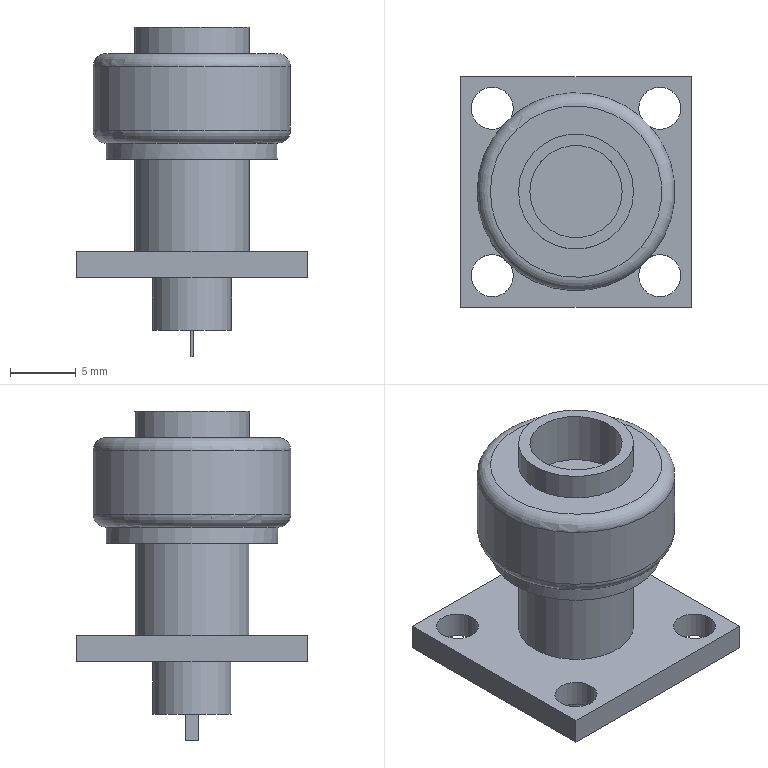Part | STEP file | N-KFD98 | 1 solid | 28 faces | box 17.5 x 17.5 x 25 mm | volume 2388 mm3 | plane 16 | cylinder 10 | torus 2 | commonest cylinder face diameters 3.2 x4 8.734 x2 6 x1 7 x1 13 x1 15 x1